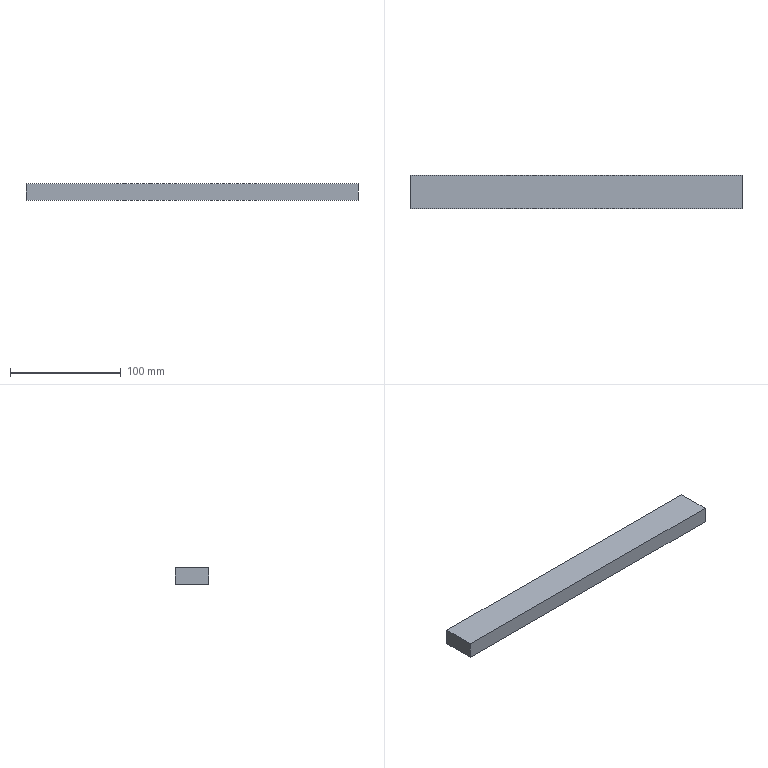Part | NX | features solid 2 | 1 solid | 6 faces | box 300 x 30 x 15 mm | volume 135000 mm3 | plane 6
STEP:
#1=CARTESIAN_POINT('',(822.5,150.,-54.));
#2=VERTEX_POINT('',#1);
#3=CARTESIAN_POINT('',(822.5,120.,-54.));
#4=VERTEX_POINT('',#3);
#5=CARTESIAN_POINT('',(822.5,0.,-54.));
#6=DIRECTION('',(0.,-1.,0.));
#7=VECTOR('',#6,1000.);
#8=LINE('',#5,#7);
#9=EDGE_CURVE('',#2,#4,#8,.T.);
#10=ORIENTED_EDGE('',*,*,#9,.T.);
#11=CARTESIAN_POINT('',(822.5,120.,-69.));
#12=VERTEX_POINT('',#11);
#13=CARTESIAN_POINT('',(822.5,120.,-69.));
#14=DIRECTION('',(0.,0.,-1.));
#15=VECTOR('',#14,1000.);
#16=LINE('',#13,#15);
#17=EDGE_CURVE('',#12,#4,#16,.F.);
#18=ORIENTED_EDGE('',*,*,#17,.F.);
#19=CARTESIAN_POINT('',(822.5,150.,-69.));
#20=VERTEX_POINT('',#19);
#21=CARTESIAN_POINT('',(822.5,0.,-69.));
#22=DIRECTION('',(0.,1.,0.));
#23=VECTOR('',#22,1000.);
#24=LINE('',#21,#23);
#25=EDGE_CURVE('',#20,#12,#24,.F.);
#26=ORIENTED_EDGE('',*,*,#25,.F.);
#27=CARTESIAN_POINT('',(822.5,150.,-69.));
#28=DIRECTION('',(0.,0.,-1.));
#29=VECTOR('',#28,1000.);
#30=LINE('',#27,#29);
#31=EDGE_CURVE('',#20,#2,#30,.F.);
#32=ORIENTED_EDGE('',*,*,#31,.T.);
#33=EDGE_LOOP('',(#10,#18,#26,#32));
#34=FACE_BOUND('',#33,.T.);
#35=CARTESIAN_POINT('',(822.5,0.,-69.));
#36=DIRECTION('',(1.,0.,0.));
#37=DIRECTION('',(0.,0.,1.));
#38=AXIS2_PLACEMENT_3D('',#35,#36,#37);
#39=PLANE('',#38);
#40=ADVANCED_FACE('',(#34),#39,.T.);
#41=ORIENTED_EDGE('',*,*,#25,.T.);
#42=CARTESIAN_POINT('',(522.5,120.,-69.));
#43=VERTEX_POINT('',#42);
#44=CARTESIAN_POINT('',(792.5,120.,-69.));
#45=DIRECTION('',(-1.,0.,0.));
#46=VECTOR('',#45,1000.);
#47=LINE('',#44,#46);
#48=EDGE_CURVE('',#12,#43,#47,.T.);
#49=ORIENTED_EDGE('',*,*,#48,.T.);
#50=CARTESIAN_POINT('',(522.5,150.,-69.));
#51=VERTEX_POINT('',#50);
#52=CARTESIAN_POINT('',(522.5,0.,-69.));
#53=DIRECTION('',(0.,-1.,0.));
#54=VECTOR('',#53,1000.);
#55=LINE('',#52,#54);
#56=EDGE_CURVE('',#51,#43,#55,.T.);
#57=ORIENTED_EDGE('',*,*,#56,.F.);
#58=CARTESIAN_POINT('',(792.5,150.,-69.));
#59=DIRECTION('',(-1.,0.,0.));
#60=VECTOR('',#59,1000.);
#61=LINE('',#58,#60);
#62=EDGE_CURVE('',#20,#51,#61,.T.);
#63=ORIENTED_EDGE('',*,*,#62,.F.);
#64=EDGE_LOOP('',(#41,#49,#57,#63));
#65=FACE_BOUND('',#64,.T.);
#66=CARTESIAN_POINT('',(792.5,0.,-69.));
#67=DIRECTION('',(0.,0.,1.));
#68=DIRECTION('',(-1.,0.,0.));
#69=AXIS2_PLACEMENT_3D('',#66,#67,#68);
#70=PLANE('',#69);
#71=ADVANCED_FACE('',(#65),#70,.F.);
#72=ORIENTED_EDGE('',*,*,#56,.T.);
#73=CARTESIAN_POINT('',(522.5,120.,-54.));
#74=VERTEX_POINT('',#73);
#75=CARTESIAN_POINT('',(522.5,120.,-69.));
#76=DIRECTION('',(0.,0.,1.));
#77=VECTOR('',#76,1000.);
#78=LINE('',#75,#77);
#79=EDGE_CURVE('',#43,#74,#78,.T.);
#80=ORIENTED_EDGE('',*,*,#79,.T.);
#81=CARTESIAN_POINT('',(522.5,150.,-54.));
#82=VERTEX_POINT('',#81);
#83=CARTESIAN_POINT('',(522.5,0.,-54.));
#84=DIRECTION('',(0.,1.,0.));
#85=VECTOR('',#84,1000.);
#86=LINE('',#83,#85);
#87=EDGE_CURVE('',#82,#74,#86,.F.);
#88=ORIENTED_EDGE('',*,*,#87,.F.);
#89=CARTESIAN_POINT('',(522.5,150.,-69.));
#90=DIRECTION('',(0.,0.,1.));
#91=VECTOR('',#90,1000.);
#92=LINE('',#89,#91);
#93=EDGE_CURVE('',#51,#82,#92,.T.);
#94=ORIENTED_EDGE('',*,*,#93,.F.);
#95=EDGE_LOOP('',(#72,#80,#88,#94));
#96=FACE_BOUND('',#95,.T.);
#97=CARTESIAN_POINT('',(522.5,0.,-84.));
#98=DIRECTION('',(1.,0.,0.));
#99=DIRECTION('',(0.,0.,1.));
#100=AXIS2_PLACEMENT_3D('',#97,#98,#99);
#101=PLANE('',#100);
#102=ADVANCED_FACE('',(#96),#101,.F.);
#103=CARTESIAN_POINT('',(792.5,150.,-54.));
#104=DIRECTION('',(1.,0.,0.));
#105=VECTOR('',#104,1000.);
#106=LINE('',#103,#105);
#107=EDGE_CURVE('',#2,#82,#106,.F.);
#108=ORIENTED_EDGE('',*,*,#107,.T.);
#109=ORIENTED_EDGE('',*,*,#87,.T.);
#110=CARTESIAN_POINT('',(792.5,120.,-54.));
#111=DIRECTION('',(1.,0.,0.));
#112=VECTOR('',#111,1000.);
#113=LINE('',#110,#112);
#114=EDGE_CURVE('',#4,#74,#113,.F.);
#115=ORIENTED_EDGE('',*,*,#114,.F.);
#116=ORIENTED_EDGE('',*,*,#9,.F.);
#117=EDGE_LOOP('',(#108,#109,#115,#116));
#118=FACE_BOUND('',#117,.T.);
#119=CARTESIAN_POINT('',(792.5,0.,-54.));
#120=DIRECTION('',(0.,0.,1.));
#121=DIRECTION('',(-1.,0.,0.));
#122=AXIS2_PLACEMENT_3D('',#119,#120,#121);
#123=PLANE('',#122);
#124=ADVANCED_FACE('',(#118),#123,.T.);
#125=ORIENTED_EDGE('',*,*,#79,.F.);
#126=ORIENTED_EDGE('',*,*,#48,.F.);
#127=ORIENTED_EDGE('',*,*,#17,.T.);
#128=ORIENTED_EDGE('',*,*,#114,.T.);
#129=EDGE_LOOP('',(#125,#126,#127,#128));
#130=FACE_BOUND('',#129,.T.);
#131=CARTESIAN_POINT('',(792.5,120.,-69.));
#132=DIRECTION('',(0.,-1.,0.));
#133=DIRECTION('',(0.,0.,-1.));
#134=AXIS2_PLACEMENT_3D('',#131,#132,#133);
#135=PLANE('',#134);
#136=ADVANCED_FACE('',(#130),#135,.T.);
#137=ORIENTED_EDGE('',*,*,#93,.T.);
#138=ORIENTED_EDGE('',*,*,#107,.F.);
#139=ORIENTED_EDGE('',*,*,#31,.F.);
#140=ORIENTED_EDGE('',*,*,#62,.T.);
#141=EDGE_LOOP('',(#137,#138,#139,#140));
#142=FACE_BOUND('',#141,.T.);
#143=CARTESIAN_POINT('',(792.5,150.,-69.));
#144=DIRECTION('',(0.,-1.,0.));
#145=DIRECTION('',(0.,0.,-1.));
#146=AXIS2_PLACEMENT_3D('',#143,#144,#145);
#147=PLANE('',#146);
#148=ADVANCED_FACE('',(#142),#147,.F.);
#149=CLOSED_SHELL('',(#40,#71,#102,#124,#136,#148));
#150=MANIFOLD_SOLID_BREP('',#149);
#151=(LENGTH_UNIT()NAMED_UNIT(*)SI_UNIT(.MILLI.,.METRE.));
#152=UNCERTAINTY_MEASURE_WITH_UNIT(LENGTH_MEASURE(0.00001),#151,'','');
#153=(NAMED_UNIT(*)PLANE_ANGLE_UNIT()SI_UNIT($,.RADIAN.));
#154=(NAMED_UNIT(*)SI_UNIT($,.STERADIAN.)SOLID_ANGLE_UNIT());
#155=(GEOMETRIC_REPRESENTATION_CONTEXT(3)GLOBAL_UNCERTAINTY_ASSIGNED_CONTEXT((#152))GLOBAL_UNIT_ASSIGNED_CONTEXT((#151,#153,#154))REPRESENTATION_CONTEXT('',''));
#156=ADVANCED_BREP_SHAPE_REPRESENTATION('',(#150),#155);